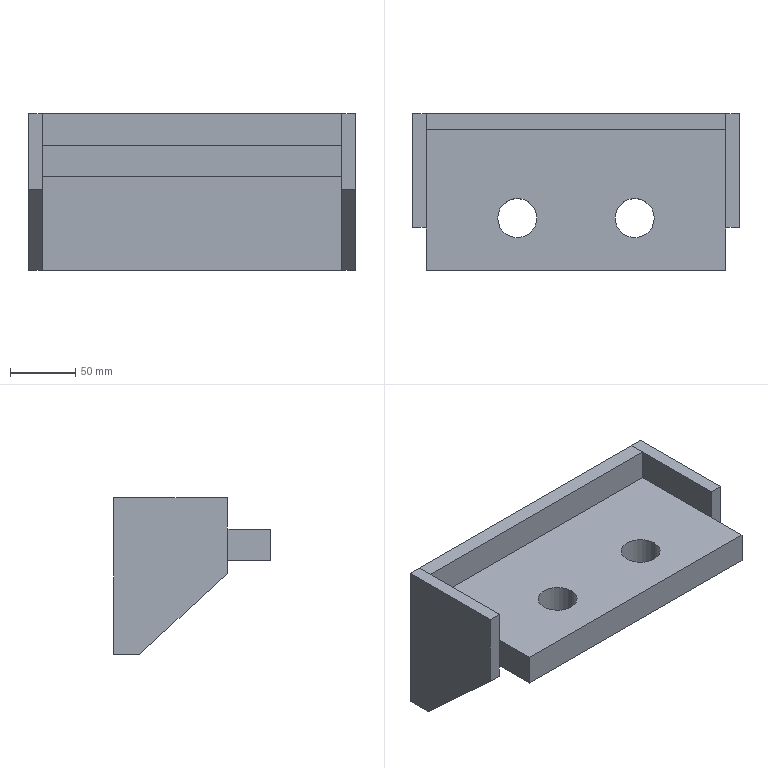Part | STEP file | Counterweight hanging seat | 4 solids | 30 faces | box 250 x 120 x 120 mm | volume 1060691 mm3 | plane 26 | cylinder 4 | commonest cylinder face diameters 30 x4